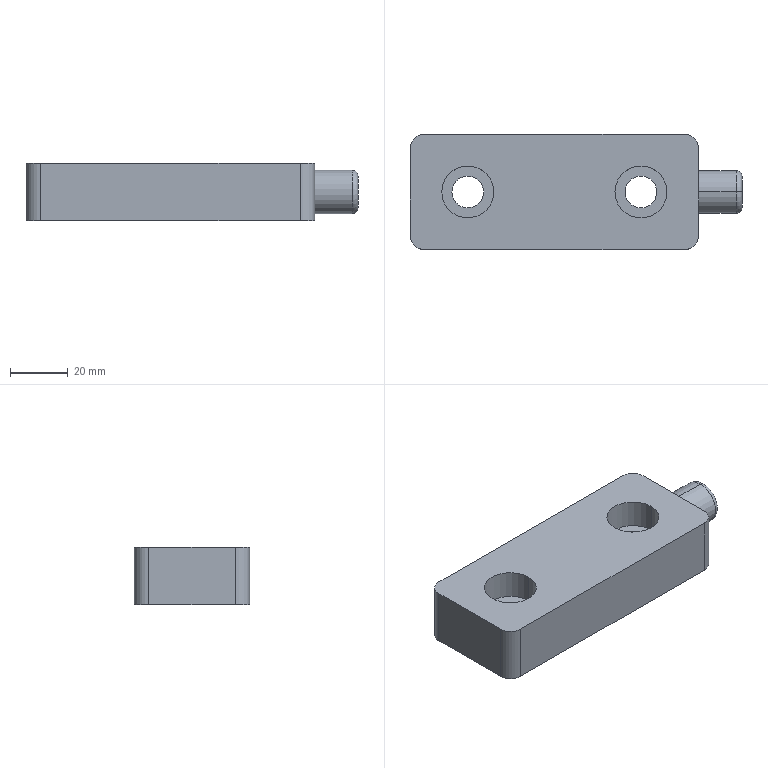Part | SolidWorks | features Fillet 2, ICE 2, Extrusion 1 | 1 solid | 25 faces | box 115 x 40 x 20 mm | volume 75193 mm3 | cylinder 14 | plane 9 | torus 2 | commonest cylinder face diameters 10 x4 11 x4 18 x4 15 x2
STEP:
#1=CARTESIAN_POINT('',(-39.,0.,0.));
#2=VERTEX_POINT('',#1);
#3=CARTESIAN_POINT('',(-21.,0.,0.));
#4=VERTEX_POINT('',#3);
#5=CARTESIAN_POINT('',(-30.,0.,0.));
#6=DIRECTION('',(0.,0.,1.));
#7=DIRECTION('',(1.,0.,0.));
#8=AXIS2_PLACEMENT_3D('',#5,#6,#7);
#9=CIRCLE('',#8,9.);
#10=EDGE_CURVE('',#2,#4,#9,.T.);
#11=ORIENTED_EDGE('',*,*,#10,.F.);
#12=CARTESIAN_POINT('',(-39.,0.,10.));
#13=VERTEX_POINT('',#12);
#14=CARTESIAN_POINT('',(-39.,0.,0.));
#15=DIRECTION('',(0.,0.,1.));
#16=VECTOR('',#15,1000.);
#17=LINE('',#14,#16);
#18=EDGE_CURVE('',#2,#13,#17,.T.);
#19=ORIENTED_EDGE('',*,*,#18,.T.);
#20=CARTESIAN_POINT('',(-21.,0.,10.));
#21=VERTEX_POINT('',#20);
#22=CARTESIAN_POINT('',(-30.,0.,10.));
#23=DIRECTION('',(0.,0.,1.));
#24=DIRECTION('',(1.,0.,0.));
#25=AXIS2_PLACEMENT_3D('',#22,#23,#24);
#26=CIRCLE('',#25,9.);
#27=EDGE_CURVE('',#13,#21,#26,.T.);
#28=ORIENTED_EDGE('',*,*,#27,.T.);
#29=CARTESIAN_POINT('',(-21.,0.,0.));
#30=DIRECTION('',(0.,0.,1.));
#31=VECTOR('',#30,1000.);
#32=LINE('',#29,#31);
#33=EDGE_CURVE('',#4,#21,#32,.T.);
#34=ORIENTED_EDGE('',*,*,#33,.F.);
#35=EDGE_LOOP('',(#11,#19,#28,#34));
#36=FACE_OUTER_BOUND('',#35,.T.);
#37=CARTESIAN_POINT('',(-30.,0.,0.));
#38=DIRECTION('',(0.,0.,1.));
#39=DIRECTION('',(1.,0.,0.));
#40=AXIS2_PLACEMENT_3D('',#37,#38,#39);
#41=CYLINDRICAL_SURFACE('',#40,9.);
#42=ADVANCED_FACE('',(#36),#41,.F.);
#43=CARTESIAN_POINT('',(21.,0.,0.));
#44=VERTEX_POINT('',#43);
#45=CARTESIAN_POINT('',(39.,0.,0.));
#46=VERTEX_POINT('',#45);
#47=CARTESIAN_POINT('',(30.,0.,0.));
#48=DIRECTION('',(0.,0.,1.));
#49=DIRECTION('',(1.,0.,0.));
#50=AXIS2_PLACEMENT_3D('',#47,#48,#49);
#51=CIRCLE('',#50,9.);
#52=EDGE_CURVE('',#44,#46,#51,.T.);
#53=ORIENTED_EDGE('',*,*,#52,.F.);
#54=CARTESIAN_POINT('',(21.,0.,10.));
#55=VERTEX_POINT('',#54);
#56=CARTESIAN_POINT('',(21.,0.,0.));
#57=DIRECTION('',(0.,0.,1.));
#58=VECTOR('',#57,1000.);
#59=LINE('',#56,#58);
#60=EDGE_CURVE('',#44,#55,#59,.T.);
#61=ORIENTED_EDGE('',*,*,#60,.T.);
#62=CARTESIAN_POINT('',(39.,0.,10.));
#63=VERTEX_POINT('',#62);
#64=CARTESIAN_POINT('',(30.,0.,10.));
#65=DIRECTION('',(0.,0.,1.));
#66=DIRECTION('',(1.,0.,0.));
#67=AXIS2_PLACEMENT_3D('',#64,#65,#66);
#68=CIRCLE('',#67,9.);
#69=EDGE_CURVE('',#55,#63,#68,.T.);
#70=ORIENTED_EDGE('',*,*,#69,.T.);
#71=CARTESIAN_POINT('',(39.,0.,0.));
#72=DIRECTION('',(0.,0.,1.));
#73=VECTOR('',#72,1000.);
#74=LINE('',#71,#73);
#75=EDGE_CURVE('',#46,#63,#74,.T.);
#76=ORIENTED_EDGE('',*,*,#75,.F.);
#77=EDGE_LOOP('',(#53,#61,#70,#76));
#78=FACE_OUTER_BOUND('',#77,.T.);
#79=CARTESIAN_POINT('',(30.,0.,0.));
#80=DIRECTION('',(0.,0.,1.));
#81=DIRECTION('',(1.,0.,0.));
#82=AXIS2_PLACEMENT_3D('',#79,#80,#81);
#83=CYLINDRICAL_SURFACE('',#82,9.);
#84=ADVANCED_FACE('',(#78),#83,.F.);
#85=CARTESIAN_POINT('',(63.,0.,7.5));
#86=VERTEX_POINT('',#85);
#87=CARTESIAN_POINT('',(63.,0.,-7.5));
#88=VERTEX_POINT('',#87);
#89=CARTESIAN_POINT('',(63.,0.,0.));
#90=DIRECTION('',(-1.,0.,0.));
#91=DIRECTION('',(0.,0.,-1.));
#92=AXIS2_PLACEMENT_3D('',#89,#90,#91);
#93=CIRCLE('',#92,7.5);
#94=EDGE_CURVE('',#86,#88,#93,.T.);
#95=ORIENTED_EDGE('',*,*,#94,.F.);
#96=CARTESIAN_POINT('',(65.,0.,5.5));
#97=VERTEX_POINT('',#96);
#98=CARTESIAN_POINT('',(63.,0.,5.5));
#99=DIRECTION('',(0.,1.,0.));
#100=DIRECTION('',(0.,0.,1.));
#101=AXIS2_PLACEMENT_3D('',#98,#99,#100);
#102=CIRCLE('',#101,2.);
#103=EDGE_CURVE('',#86,#97,#102,.T.);
#104=ORIENTED_EDGE('',*,*,#103,.T.);
#105=CARTESIAN_POINT('',(65.,0.,-5.5));
#106=VERTEX_POINT('',#105);
#107=CARTESIAN_POINT('',(65.,0.,0.));
#108=DIRECTION('',(1.,0.,0.));
#109=DIRECTION('',(0.,0.,-1.));
#110=AXIS2_PLACEMENT_3D('',#107,#108,#109);
#111=CIRCLE('',#110,5.5);
#112=EDGE_CURVE('',#106,#97,#111,.T.);
#113=ORIENTED_EDGE('',*,*,#112,.F.);
#114=CARTESIAN_POINT('',(63.,0.,-5.5));
#115=DIRECTION('',(0.,-1.,0.));
#116=DIRECTION('',(0.,0.,-1.));
#117=AXIS2_PLACEMENT_3D('',#114,#115,#116);
#118=CIRCLE('',#117,2.);
#119=EDGE_CURVE('',#88,#106,#118,.T.);
#120=ORIENTED_EDGE('',*,*,#119,.F.);
#121=EDGE_LOOP('',(#95,#104,#113,#120));
#122=FACE_OUTER_BOUND('',#121,.T.);
#123=CARTESIAN_POINT('',(63.,0.,0.));
#124=DIRECTION('',(1.,0.,0.));
#125=DIRECTION('',(0.,0.,-1.));
#126=AXIS2_PLACEMENT_3D('',#123,#124,#125);
#127=TOROIDAL_SURFACE('',#126,5.5,2.);
#128=ADVANCED_FACE('',(#122),#127,.T.);
#129=ORIENTED_EDGE('',*,*,#94,.T.);
#130=CARTESIAN_POINT('',(50.,0.,-7.5));
#131=VERTEX_POINT('',#130);
#132=CARTESIAN_POINT('',(65.,0.,-7.5));
#133=DIRECTION('',(-1.,0.,0.));
#134=VECTOR('',#133,1000.);
#135=LINE('',#132,#134);
#136=EDGE_CURVE('',#88,#131,#135,.T.);
#137=ORIENTED_EDGE('',*,*,#136,.T.);
#138=CARTESIAN_POINT('',(50.,0.,7.5));
#139=VERTEX_POINT('',#138);
#140=CARTESIAN_POINT('',(50.,0.,0.));
#141=DIRECTION('',(1.,0.,0.));
#142=DIRECTION('',(0.,0.,-1.));
#143=AXIS2_PLACEMENT_3D('',#140,#141,#142);
#144=CIRCLE('',#143,7.5);
#145=EDGE_CURVE('',#131,#139,#144,.T.);
#146=ORIENTED_EDGE('',*,*,#145,.T.);
#147=CARTESIAN_POINT('',(65.,0.,7.5));
#148=DIRECTION('',(-1.,0.,0.));
#149=VECTOR('',#148,1000.);
#150=LINE('',#147,#149);
#151=EDGE_CURVE('',#86,#139,#150,.T.);
#152=ORIENTED_EDGE('',*,*,#151,.F.);
#153=EDGE_LOOP('',(#129,#137,#146,#152));
#154=FACE_OUTER_BOUND('',#153,.T.);
#155=CARTESIAN_POINT('',(65.,0.,0.));
#156=DIRECTION('',(-1.,0.,0.));
#157=DIRECTION('',(0.,0.,1.));
#158=AXIS2_PLACEMENT_3D('',#155,#156,#157);
#159=CYLINDRICAL_SURFACE('',#158,7.5);
#160=ADVANCED_FACE('',(#154),#159,.T.);
#161=CARTESIAN_POINT('',(24.5,0.,0.));
#162=VERTEX_POINT('',#161);
#163=CARTESIAN_POINT('',(35.5,0.,0.));
#164=VERTEX_POINT('',#163);
#165=CARTESIAN_POINT('',(30.,0.,0.));
#166=DIRECTION('',(0.,0.,1.));
#167=DIRECTION('',(1.,0.,0.));
#168=AXIS2_PLACEMENT_3D('',#165,#166,#167);
#169=CIRCLE('',#168,5.5);
#170=EDGE_CURVE('',#162,#164,#169,.T.);
#171=ORIENTED_EDGE('',*,*,#170,.T.);
#172=CARTESIAN_POINT('',(35.5,0.,-10.));
#173=VERTEX_POINT('',#172);
#174=CARTESIAN_POINT('',(35.5,0.,10.));
#175=DIRECTION('',(0.,0.,-1.));
#176=VECTOR('',#175,1000.);
#177=LINE('',#174,#176);
#178=EDGE_CURVE('',#164,#173,#177,.T.);
#179=ORIENTED_EDGE('',*,*,#178,.T.);
#180=CARTESIAN_POINT('',(24.5,0.,-10.));
#181=VERTEX_POINT('',#180);
#182=CARTESIAN_POINT('',(30.,0.,-10.));
#183=DIRECTION('',(0.,0.,1.));
#184=DIRECTION('',(1.,0.,0.));
#185=AXIS2_PLACEMENT_3D('',#182,#183,#184);
#186=CIRCLE('',#185,5.5);
#187=EDGE_CURVE('',#181,#173,#186,.T.);
#188=ORIENTED_EDGE('',*,*,#187,.F.);
#189=CARTESIAN_POINT('',(24.5,0.,10.));
#190=DIRECTION('',(0.,0.,-1.));
#191=VECTOR('',#190,1000.);
#192=LINE('',#189,#191);
#193=EDGE_CURVE('',#162,#181,#192,.T.);
#194=ORIENTED_EDGE('',*,*,#193,.F.);
#195=EDGE_LOOP('',(#171,#179,#188,#194));
#196=FACE_OUTER_BOUND('',#195,.T.);
#197=CARTESIAN_POINT('',(30.,0.,10.));
#198=DIRECTION('',(0.,0.,-1.));
#199=DIRECTION('',(-1.,0.,0.));
#200=AXIS2_PLACEMENT_3D('',#197,#198,#199);
#201=CYLINDRICAL_SURFACE('',#200,5.5);
#202=ADVANCED_FACE('',(#196),#201,.F.);
#203=CARTESIAN_POINT('',(-35.5,0.,0.));
#204=VERTEX_POINT('',#203);
#205=CARTESIAN_POINT('',(-24.5,0.,0.));
#206=VERTEX_POINT('',#205);
#207=CARTESIAN_POINT('',(-30.,0.,0.));
#208=DIRECTION('',(0.,0.,1.));
#209=DIRECTION('',(1.,0.,0.));
#210=AXIS2_PLACEMENT_3D('',#207,#208,#209);
#211=CIRCLE('',#210,5.5);
#212=EDGE_CURVE('',#204,#206,#211,.T.);
#213=ORIENTED_EDGE('',*,*,#212,.T.);
#214=CARTESIAN_POINT('',(-24.5,0.,-10.));
#215=VERTEX_POINT('',#214);
#216=CARTESIAN_POINT('',(-24.5,0.,10.));
#217=DIRECTION('',(0.,0.,-1.));
#218=VECTOR('',#217,1000.);
#219=LINE('',#216,#218);
#220=EDGE_CURVE('',#206,#215,#219,.T.);
#221=ORIENTED_EDGE('',*,*,#220,.T.);
#222=CARTESIAN_POINT('',(-35.5,0.,-10.));
#223=VERTEX_POINT('',#222);
#224=CARTESIAN_POINT('',(-30.,0.,-10.));
#225=DIRECTION('',(0.,0.,1.));
#226=DIRECTION('',(1.,0.,0.));
#227=AXIS2_PLACEMENT_3D('',#224,#225,#226);
#228=CIRCLE('',#227,5.5);
#229=EDGE_CURVE('',#223,#215,#228,.T.);
#230=ORIENTED_EDGE('',*,*,#229,.F.);
#231=CARTESIAN_POINT('',(-35.5,0.,10.));
#232=DIRECTION('',(0.,0.,-1.));
#233=VECTOR('',#232,1000.);
#234=LINE('',#231,#233);
#235=EDGE_CURVE('',#204,#223,#234,.T.);
#236=ORIENTED_EDGE('',*,*,#235,.F.);
#237=EDGE_LOOP('',(#213,#221,#230,#236));
#238=FACE_OUTER_BOUND('',#237,.T.);
#239=CARTESIAN_POINT('',(-30.,0.,10.));
#240=DIRECTION('',(0.,0.,-1.));
#241=DIRECTION('',(-1.,0.,0.));
#242=AXIS2_PLACEMENT_3D('',#239,#240,#241);
#243=CYLINDRICAL_SURFACE('',#242,5.5);
#244=ADVANCED_FACE('',(#238),#243,.F.);
#245=ORIENTED_EDGE('',*,*,#220,.F.);
#246=CARTESIAN_POINT('',(-30.,0.,0.));
#247=DIRECTION('',(0.,0.,1.));
#248=DIRECTION('',(1.,0.,0.));
#249=AXIS2_PLACEMENT_3D('',#246,#247,#248);
#250=CIRCLE('',#249,5.5);
#251=EDGE_CURVE('',#206,#204,#250,.T.);
#252=ORIENTED_EDGE('',*,*,#251,.T.);
#253=ORIENTED_EDGE('',*,*,#235,.T.);
#254=CARTESIAN_POINT('',(-30.,0.,-10.));
#255=DIRECTION('',(0.,0.,1.));
#256=DIRECTION('',(1.,0.,0.));
#257=AXIS2_PLACEMENT_3D('',#254,#255,#256);
#258=CIRCLE('',#257,5.5);
#259=EDGE_CURVE('',#215,#223,#258,.T.);
#260=ORIENTED_EDGE('',*,*,#259,.F.);
#261=EDGE_LOOP('',(#245,#252,#253,#260));
#262=FACE_OUTER_BOUND('',#261,.T.);
#263=CARTESIAN_POINT('',(-30.,0.,10.));
#264=DIRECTION('',(0.,0.,-1.));
#265=DIRECTION('',(-1.,0.,0.));
#266=AXIS2_PLACEMENT_3D('',#263,#264,#265);
#267=CYLINDRICAL_SURFACE('',#266,5.5);
#268=ADVANCED_FACE('',(#262),#267,.F.);
#269=ORIENTED_EDGE('',*,*,#178,.F.);
#270=CARTESIAN_POINT('',(30.,0.,0.));
#271=DIRECTION('',(0.,0.,1.));
#272=DIRECTION('',(1.,0.,0.));
#273=AXIS2_PLACEMENT_3D('',#270,#271,#272);
#274=CIRCLE('',#273,5.5);
#275=EDGE_CURVE('',#164,#162,#274,.T.);
#276=ORIENTED_EDGE('',*,*,#275,.T.);
#277=ORIENTED_EDGE('',*,*,#193,.T.);
#278=CARTESIAN_POINT('',(30.,0.,-10.));
#279=DIRECTION('',(0.,0.,1.));
#280=DIRECTION('',(1.,0.,0.));
#281=AXIS2_PLACEMENT_3D('',#278,#279,#280);
#282=CIRCLE('',#281,5.5);
#283=EDGE_CURVE('',#173,#181,#282,.T.);
#284=ORIENTED_EDGE('',*,*,#283,.F.);
#285=EDGE_LOOP('',(#269,#276,#277,#284));
#286=FACE_OUTER_BOUND('',#285,.T.);
#287=CARTESIAN_POINT('',(30.,0.,10.));
#288=DIRECTION('',(0.,0.,-1.));
#289=DIRECTION('',(-1.,0.,0.));
#290=AXIS2_PLACEMENT_3D('',#287,#288,#289);
#291=CYLINDRICAL_SURFACE('',#290,5.5);
#292=ADVANCED_FACE('',(#286),#291,.F.);
#293=CARTESIAN_POINT('',(-30.,0.,10.));
#294=DIRECTION('',(0.,0.,1.));
#295=DIRECTION('',(1.,0.,0.));
#296=AXIS2_PLACEMENT_3D('',#293,#294,#295);
#297=CIRCLE('',#296,9.);
#298=EDGE_CURVE('',#21,#13,#297,.T.);
#299=ORIENTED_EDGE('',*,*,#298,.F.);
#300=ORIENTED_EDGE('',*,*,#27,.F.);
#301=EDGE_LOOP('',(#299,#300));
#302=FACE_BOUND('',#301,.T.);
#303=CARTESIAN_POINT('',(30.,0.,10.));
#304=DIRECTION('',(0.,0.,1.));
#305=DIRECTION('',(1.,0.,0.));
#306=AXIS2_PLACEMENT_3D('',#303,#304,#305);
#307=CIRCLE('',#306,9.);
#308=EDGE_CURVE('',#63,#55,#307,.T.);
#309=ORIENTED_EDGE('',*,*,#308,.F.);
#310=ORIENTED_EDGE('',*,*,#69,.F.);
#311=EDGE_LOOP('',(#309,#310));
#312=FACE_BOUND('',#311,.T.);
#313=CARTESIAN_POINT('',(50.,-15.,10.));
#314=VERTEX_POINT('',#313);
#315=CARTESIAN_POINT('',(50.,15.,10.));
#316=VERTEX_POINT('',#315);
#317=CARTESIAN_POINT('',(50.,-20.,10.));
#318=DIRECTION('',(0.,1.,0.));
#319=VECTOR('',#318,1000.);
#320=LINE('',#317,#319);
#321=EDGE_CURVE('',#314,#316,#320,.T.);
#322=ORIENTED_EDGE('',*,*,#321,.T.);
#323=CARTESIAN_POINT('',(45.,20.,10.));
#324=VERTEX_POINT('',#323);
#325=CARTESIAN_POINT('',(45.,15.,10.));
#326=DIRECTION('',(0.,0.,1.));
#327=DIRECTION('',(-1.,0.,0.));
#328=AXIS2_PLACEMENT_3D('',#325,#326,#327);
#329=CIRCLE('',#328,5.);
#330=EDGE_CURVE('',#316,#324,#329,.T.);
#331=ORIENTED_EDGE('',*,*,#330,.T.);
#332=CARTESIAN_POINT('',(-45.,20.,10.));
#333=VERTEX_POINT('',#332);
#334=CARTESIAN_POINT('',(-50.,20.,10.));
#335=DIRECTION('',(-1.,0.,0.));
#336=VECTOR('',#335,1000.);
#337=LINE('',#334,#336);
#338=EDGE_CURVE('',#324,#333,#337,.T.);
#339=ORIENTED_EDGE('',*,*,#338,.T.);
#340=CARTESIAN_POINT('',(-50.,15.,10.));
#341=VERTEX_POINT('',#340);
#342=CARTESIAN_POINT('',(-45.,15.,10.));
#343=DIRECTION('',(0.,0.,1.));
#344=DIRECTION('',(-1.,0.,0.));
#345=AXIS2_PLACEMENT_3D('',#342,#343,#344);
#346=CIRCLE('',#345,5.);
#347=EDGE_CURVE('',#333,#341,#346,.T.);
#348=ORIENTED_EDGE('',*,*,#347,.T.);
#349=CARTESIAN_POINT('',(-50.,-15.,10.));
#350=VERTEX_POINT('',#349);
#351=CARTESIAN_POINT('',(-50.,-20.,10.));
#352=DIRECTION('',(0.,-1.,0.));
#353=VECTOR('',#352,1000.);
#354=LINE('',#351,#353);
#355=EDGE_CURVE('',#341,#350,#354,.T.);
#356=ORIENTED_EDGE('',*,*,#355,.T.);
#357=CARTESIAN_POINT('',(-45.,-20.,10.));
#358=VERTEX_POINT('',#357);
#359=CARTESIAN_POINT('',(-45.,-15.,10.));
#360=DIRECTION('',(0.,0.,1.));
#361=DIRECTION('',(-1.,0.,0.));
#362=AXIS2_PLACEMENT_3D('',#359,#360,#361);
#363=CIRCLE('',#362,5.);
#364=EDGE_CURVE('',#350,#358,#363,.T.);
#365=ORIENTED_EDGE('',*,*,#364,.T.);
#366=CARTESIAN_POINT('',(45.,-20.,10.));
#367=VERTEX_POINT('',#366);
#368=CARTESIAN_POINT('',(-50.,-20.,10.));
#369=DIRECTION('',(1.,0.,0.));
#370=VECTOR('',#369,1000.);
#371=LINE('',#368,#370);
#372=EDGE_CURVE('',#358,#367,#371,.T.);
#373=ORIENTED_EDGE('',*,*,#372,.T.);
#374=CARTESIAN_POINT('',(45.,-15.,10.));
#375=DIRECTION('',(0.,0.,1.));
#376=DIRECTION('',(-1.,0.,0.));
#377=AXIS2_PLACEMENT_3D('',#374,#375,#376);
#378=CIRCLE('',#377,5.);
#379=EDGE_CURVE('',#367,#314,#378,.T.);
#380=ORIENTED_EDGE('',*,*,#379,.T.);
#381=EDGE_LOOP('',(#322,#331,#339,#348,#356,#365,#373,#380));
#382=FACE_OUTER_BOUND('',#381,.T.);
#383=CARTESIAN_POINT('',(0.,0.,10.));
#384=DIRECTION('',(0.,0.,-1.));
#385=DIRECTION('',(-1.,0.,0.));
#386=AXIS2_PLACEMENT_3D('',#383,#384,#385);
#387=PLANE('',#386);
#388=ADVANCED_FACE('',(#302,#312,#382),#387,.F.);
#389=ORIENTED_EDGE('',*,*,#229,.T.);
#390=ORIENTED_EDGE('',*,*,#259,.T.);
#391=EDGE_LOOP('',(#389,#390));
#392=FACE_BOUND('',#391,.T.);
#393=CARTESIAN_POINT('',(45.,20.,-10.));
#394=VERTEX_POINT('',#393);
#395=CARTESIAN_POINT('',(-45.,20.,-10.));
#396=VERTEX_POINT('',#395);
#397=CARTESIAN_POINT('',(-50.,20.,-10.));
#398=DIRECTION('',(-1.,0.,0.));
#399=VECTOR('',#398,1000.);
#400=LINE('',#397,#399);
#401=EDGE_CURVE('',#394,#396,#400,.T.);
#402=ORIENTED_EDGE('',*,*,#401,.F.);
#403=CARTESIAN_POINT('',(50.,15.,-10.));
#404=VERTEX_POINT('',#403);
#405=CARTESIAN_POINT('',(45.,15.,-10.));
#406=DIRECTION('',(0.,0.,-1.));
#407=DIRECTION('',(-1.,0.,0.));
#408=AXIS2_PLACEMENT_3D('',#405,#406,#407);
#409=CIRCLE('',#408,5.);
#410=EDGE_CURVE('',#394,#404,#409,.T.);
#411=ORIENTED_EDGE('',*,*,#410,.T.);
#412=CARTESIAN_POINT('',(50.,-15.,-10.));
#413=VERTEX_POINT('',#412);
#414=CARTESIAN_POINT('',(50.,-20.,-10.));
#415=DIRECTION('',(0.,1.,0.));
#416=VECTOR('',#415,1000.);
#417=LINE('',#414,#416);
#418=EDGE_CURVE('',#413,#404,#417,.T.);
#419=ORIENTED_EDGE('',*,*,#418,.F.);
#420=CARTESIAN_POINT('',(45.,-20.,-10.));
#421=VERTEX_POINT('',#420);
#422=CARTESIAN_POINT('',(45.,-15.,-10.));
#423=DIRECTION('',(0.,0.,-1.));
#424=DIRECTION('',(-1.,0.,0.));
#425=AXIS2_PLACEMENT_3D('',#422,#423,#424);
#426=CIRCLE('',#425,5.);
#427=EDGE_CURVE('',#413,#421,#426,.T.);
#428=ORIENTED_EDGE('',*,*,#427,.T.);
#429=CARTESIAN_POINT('',(-45.,-20.,-10.));
#430=VERTEX_POINT('',#429);
#431=CARTESIAN_POINT('',(-50.,-20.,-10.));
#432=DIRECTION('',(1.,0.,0.));
#433=VECTOR('',#432,1000.);
#434=LINE('',#431,#433);
#435=EDGE_CURVE('',#430,#421,#434,.T.);
#436=ORIENTED_EDGE('',*,*,#435,.F.);
#437=CARTESIAN_POINT('',(-50.,-15.,-10.));
#438=VERTEX_POINT('',#437);
#439=CARTESIAN_POINT('',(-45.,-15.,-10.));
#440=DIRECTION('',(0.,0.,-1.));
#441=DIRECTION('',(-1.,0.,0.));
#442=AXIS2_PLACEMENT_3D('',#439,#440,#441);
#443=CIRCLE('',#442,5.);
#444=EDGE_CURVE('',#430,#438,#443,.T.);
#445=ORIENTED_EDGE('',*,*,#444,.T.);
#446=CARTESIAN_POINT('',(-50.,15.,-10.));
#447=VERTEX_POINT('',#446);
#448=CARTESIAN_POINT('',(-50.,-20.,-10.));
#449=DIRECTION('',(0.,-1.,0.));
#450=VECTOR('',#449,1000.);
#451=LINE('',#448,#450);
#452=EDGE_CURVE('',#447,#438,#451,.T.);
#453=ORIENTED_EDGE('',*,*,#452,.F.);
#454=CARTESIAN_POINT('',(-45.,15.,-10.));
#455=DIRECTION('',(0.,0.,-1.));
#456=DIRECTION('',(-1.,0.,0.));
#457=AXIS2_PLACEMENT_3D('',#454,#455,#456);
#458=CIRCLE('',#457,5.);
#459=EDGE_CURVE('',#447,#396,#458,.T.);
#460=ORIENTED_EDGE('',*,*,#459,.T.);
#461=EDGE_LOOP('',(#402,#411,#419,#428,#436,#445,#453,#460));
#462=FACE_OUTER_BOUND('',#461,.T.);
#463=ORIENTED_EDGE('',*,*,#187,.T.);
#464=ORIENTED_EDGE('',*,*,#283,.T.);
#465=EDGE_LOOP('',(#463,#464));
#466=FACE_BOUND('',#465,.T.);
#467=CARTESIAN_POINT('',(0.,0.,-10.));
#468=DIRECTION('',(0.,0.,-1.));
#469=DIRECTION('',(-1.,0.,0.));
#470=AXIS2_PLACEMENT_3D('',#467,#468,#469);
#471=PLANE('',#470);
#472=ADVANCED_FACE('',(#392,#462,#466),#471,.T.);
#473=CARTESIAN_POINT('',(50.,0.,0.));
#474=DIRECTION('',(1.,0.,0.));
#475=DIRECTION('',(0.,0.,-1.));
#476=AXIS2_PLACEMENT_3D('',#473,#474,#475);
#477=CIRCLE('',#476,7.5);
#478=EDGE_CURVE('',#139,#131,#477,.T.);
#479=ORIENTED_EDGE('',*,*,#478,.F.);
#480=ORIENTED_EDGE('',*,*,#145,.F.);
#481=EDGE_LOOP('',(#479,#480));
#482=FACE_BOUND('',#481,.T.);
#483=ORIENTED_EDGE('',*,*,#418,.T.);
#484=CARTESIAN_POINT('',(50.,15.,10.));
#485=DIRECTION('',(0.,0.,1.));
#486=VECTOR('',#485,1000.);
#487=LINE('',#484,#486);
#488=EDGE_CURVE('',#404,#316,#487,.T.);
#489=ORIENTED_EDGE('',*,*,#488,.T.);
#490=ORIENTED_EDGE('',*,*,#321,.F.);
#491=CARTESIAN_POINT('',(50.,-15.,10.));
#492=DIRECTION('',(0.,0.,-1.));
#493=VECTOR('',#492,1000.);
#494=LINE('',#491,#493);
#495=EDGE_CURVE('',#314,#413,#494,.T.);
#496=ORIENTED_EDGE('',*,*,#495,.T.);
#497=EDGE_LOOP('',(#483,#489,#490,#496));
#498=FACE_OUTER_BOUND('',#497,.T.);
#499=CARTESIAN_POINT('',(50.,-20.,10.));
#500=DIRECTION('',(-1.,0.,0.));
#501=DIRECTION('',(0.,0.,1.));
#502=AXIS2_PLACEMENT_3D('',#499,#500,#501);
#503=PLANE('',#502);
#504=ADVANCED_FACE('',(#482,#498),#503,.F.);
#505=ORIENTED_EDGE('',*,*,#338,.F.);
#506=CARTESIAN_POINT('',(45.,20.,10.));
#507=DIRECTION('',(0.,0.,-1.));
#508=VECTOR('',#507,1000.);
#509=LINE('',#506,#508);
#510=EDGE_CURVE('',#324,#394,#509,.T.);
#511=ORIENTED_EDGE('',*,*,#510,.T.);
#512=ORIENTED_EDGE('',*,*,#401,.T.);
#513=CARTESIAN_POINT('',(-45.,20.,10.));
#514=DIRECTION('',(0.,0.,1.));
#515=VECTOR('',#514,1000.);
#516=LINE('',#513,#515);
#517=EDGE_CURVE('',#396,#333,#516,.T.);
#518=ORIENTED_EDGE('',*,*,#517,.T.);
#519=EDGE_LOOP('',(#505,#511,#512,#518));
#520=FACE_OUTER_BOUND('',#519,.T.);
#521=CARTESIAN_POINT('',(-50.,20.,10.));
#522=DIRECTION('',(0.,-1.,0.));
#523=DIRECTION('',(0.,0.,-1.));
#524=AXIS2_PLACEMENT_3D('',#521,#522,#523);
#525=PLANE('',#524);
#526=ADVANCED_FACE('',(#520),#525,.F.);
#527=ORIENTED_EDGE('',*,*,#452,.T.);
#528=CARTESIAN_POINT('',(-50.,-15.,10.));
#529=DIRECTION('',(0.,0.,1.));
#530=VECTOR('',#529,1000.);
#531=LINE('',#528,#530);
#532=EDGE_CURVE('',#438,#350,#531,.T.);
#533=ORIENTED_EDGE('',*,*,#532,.T.);
#534=ORIENTED_EDGE('',*,*,#355,.F.);
#535=CARTESIAN_POINT('',(-50.,15.,10.));
#536=DIRECTION('',(0.,0.,-1.));
#537=VECTOR('',#536,1000.);
#538=LINE('',#535,#537);
#539=EDGE_CURVE('',#341,#447,#538,.T.);
#540=ORIENTED_EDGE('',*,*,#539,.T.);
#541=EDGE_LOOP('',(#527,#533,#534,#540));
#542=FACE_OUTER_BOUND('',#541,.T.);
#543=CARTESIAN_POINT('',(-50.,-20.,10.));
#544=DIRECTION('',(1.,0.,0.));
#545=DIRECTION('',(0.,0.,-1.));
#546=AXIS2_PLACEMENT_3D('',#543,#544,#545);
#547=PLANE('',#546);
#548=ADVANCED_FACE('',(#542),#547,.F.);
#549=ORIENTED_EDGE('',*,*,#435,.T.);
#550=CARTESIAN_POINT('',(45.,-20.,10.));
#551=DIRECTION('',(0.,0.,1.));
#552=VECTOR('',#551,1000.);
#553=LINE('',#550,#552);
#554=EDGE_CURVE('',#421,#367,#553,.T.);
#555=ORIENTED_EDGE('',*,*,#554,.T.);
#556=ORIENTED_EDGE('',*,*,#372,.F.);
#557=CARTESIAN_POINT('',(-45.,-20.,10.));
#558=DIRECTION('',(0.,0.,-1.));
#559=VECTOR('',#558,1000.);
#560=LINE('',#557,#559);
#561=EDGE_CURVE('',#358,#430,#560,.T.);
#562=ORIENTED_EDGE('',*,*,#561,.T.);
#563=EDGE_LOOP('',(#549,#555,#556,#562));
#564=FACE_OUTER_BOUND('',#563,.T.);
#565=CARTESIAN_POINT('',(-50.,-20.,10.));
#566=DIRECTION('',(0.,1.,0.));
#567=DIRECTION('',(0.,0.,1.));
#568=AXIS2_PLACEMENT_3D('',#565,#566,#567);
#569=PLANE('',#568);
#570=ADVANCED_FACE('',(#564),#569,.F.);
#571=ORIENTED_EDGE('',*,*,#136,.F.);
#572=CARTESIAN_POINT('',(63.,0.,0.));
#573=DIRECTION('',(-1.,0.,0.));
#574=DIRECTION('',(0.,0.,-1.));
#575=AXIS2_PLACEMENT_3D('',#572,#573,#574);
#576=CIRCLE('',#575,7.5);
#577=EDGE_CURVE('',#88,#86,#576,.T.);
#578=ORIENTED_EDGE('',*,*,#577,.T.);
#579=ORIENTED_EDGE('',*,*,#151,.T.);
#580=ORIENTED_EDGE('',*,*,#478,.T.);
#581=EDGE_LOOP('',(#571,#578,#579,#580));
#582=FACE_OUTER_BOUND('',#581,.T.);
#583=CARTESIAN_POINT('',(65.,0.,0.));
#584=DIRECTION('',(-1.,0.,0.));
#585=DIRECTION('',(0.,0.,1.));
#586=AXIS2_PLACEMENT_3D('',#583,#584,#585);
#587=CYLINDRICAL_SURFACE('',#586,7.5);
#588=ADVANCED_FACE('',(#582),#587,.T.);
#589=ORIENTED_EDGE('',*,*,#112,.T.);
#590=CARTESIAN_POINT('',(65.,0.,0.));
#591=DIRECTION('',(1.,0.,0.));
#592=DIRECTION('',(0.,0.,-1.));
#593=AXIS2_PLACEMENT_3D('',#590,#591,#592);
#594=CIRCLE('',#593,5.5);
#595=EDGE_CURVE('',#97,#106,#594,.T.);
#596=ORIENTED_EDGE('',*,*,#595,.T.);
#597=EDGE_LOOP('',(#589,#596));
#598=FACE_OUTER_BOUND('',#597,.T.);
#599=CARTESIAN_POINT('',(65.,0.,0.));
#600=DIRECTION('',(1.,0.,0.));
#601=DIRECTION('',(0.,0.,-1.));
#602=AXIS2_PLACEMENT_3D('',#599,#600,#601);
#603=PLANE('',#602);
#604=ADVANCED_FACE('',(#598),#603,.T.);
#605=ORIENTED_EDGE('',*,*,#103,.F.);
#606=ORIENTED_EDGE('',*,*,#577,.F.);
#607=ORIENTED_EDGE('',*,*,#119,.T.);
#608=ORIENTED_EDGE('',*,*,#595,.F.);
#609=EDGE_LOOP('',(#605,#606,#607,#608));
#610=FACE_OUTER_BOUND('',#609,.T.);
#611=CARTESIAN_POINT('',(63.,0.,0.));
#612=DIRECTION('',(1.,0.,0.));
#613=DIRECTION('',(0.,0.,-1.));
#614=AXIS2_PLACEMENT_3D('',#611,#612,#613);
#615=TOROIDAL_SURFACE('',#614,5.5,2.);
#616=ADVANCED_FACE('',(#610),#615,.T.);
#617=ORIENTED_EDGE('',*,*,#60,.F.);
#618=CARTESIAN_POINT('',(30.,0.,0.));
#619=DIRECTION('',(0.,0.,1.));
#620=DIRECTION('',(1.,0.,0.));
#621=AXIS2_PLACEMENT_3D('',#618,#619,#620);
#622=CIRCLE('',#621,9.);
#623=EDGE_CURVE('',#46,#44,#622,.T.);
#624=ORIENTED_EDGE('',*,*,#623,.F.);
#625=ORIENTED_EDGE('',*,*,#75,.T.);
#626=ORIENTED_EDGE('',*,*,#308,.T.);
#627=EDGE_LOOP('',(#617,#624,#625,#626));
#628=FACE_OUTER_BOUND('',#627,.T.);
#629=CARTESIAN_POINT('',(30.,0.,0.));
#630=DIRECTION('',(0.,0.,1.));
#631=DIRECTION('',(1.,0.,0.));
#632=AXIS2_PLACEMENT_3D('',#629,#630,#631);
#633=CYLINDRICAL_SURFACE('',#632,9.);
#634=ADVANCED_FACE('',(#628),#633,.F.);
#635=ORIENTED_EDGE('',*,*,#170,.F.);
#636=ORIENTED_EDGE('',*,*,#275,.F.);
#637=EDGE_LOOP('',(#635,#636));
#638=FACE_BOUND('',#637,.T.);
#639=ORIENTED_EDGE('',*,*,#623,.T.);
#640=ORIENTED_EDGE('',*,*,#52,.T.);
#641=EDGE_LOOP('',(#639,#640));
#642=FACE_OUTER_BOUND('',#641,.T.);
#643=CARTESIAN_POINT('',(30.,0.,0.));
#644=DIRECTION('',(0.,0.,1.));
#645=DIRECTION('',(1.,0.,0.));
#646=AXIS2_PLACEMENT_3D('',#643,#644,#645);
#647=PLANE('',#646);
#648=ADVANCED_FACE('',(#638,#642),#647,.T.);
#649=ORIENTED_EDGE('',*,*,#18,.F.);
#650=CARTESIAN_POINT('',(-30.,0.,0.));
#651=DIRECTION('',(0.,0.,1.));
#652=DIRECTION('',(1.,0.,0.));
#653=AXIS2_PLACEMENT_3D('',#650,#651,#652);
#654=CIRCLE('',#653,9.);
#655=EDGE_CURVE('',#4,#2,#654,.T.);
#656=ORIENTED_EDGE('',*,*,#655,.F.);
#657=ORIENTED_EDGE('',*,*,#33,.T.);
#658=ORIENTED_EDGE('',*,*,#298,.T.);
#659=EDGE_LOOP('',(#649,#656,#657,#658));
#660=FACE_OUTER_BOUND('',#659,.T.);
#661=CARTESIAN_POINT('',(-30.,0.,0.));
#662=DIRECTION('',(0.,0.,1.));
#663=DIRECTION('',(1.,0.,0.));
#664=AXIS2_PLACEMENT_3D('',#661,#662,#663);
#665=CYLINDRICAL_SURFACE('',#664,9.);
#666=ADVANCED_FACE('',(#660),#665,.F.);
#667=ORIENTED_EDGE('',*,*,#212,.F.);
#668=ORIENTED_EDGE('',*,*,#251,.F.);
#669=EDGE_LOOP('',(#667,#668));
#670=FACE_BOUND('',#669,.T.);
#671=ORIENTED_EDGE('',*,*,#655,.T.);
#672=ORIENTED_EDGE('',*,*,#10,.T.);
#673=EDGE_LOOP('',(#671,#672));
#674=FACE_OUTER_BOUND('',#673,.T.);
#675=CARTESIAN_POINT('',(-30.,0.,0.));
#676=DIRECTION('',(0.,0.,1.));
#677=DIRECTION('',(1.,0.,0.));
#678=AXIS2_PLACEMENT_3D('',#675,#676,#677);
#679=PLANE('',#678);
#680=ADVANCED_FACE('',(#670,#674),#679,.T.);
#681=ORIENTED_EDGE('',*,*,#330,.F.);
#682=ORIENTED_EDGE('',*,*,#488,.F.);
#683=ORIENTED_EDGE('',*,*,#410,.F.);
#684=ORIENTED_EDGE('',*,*,#510,.F.);
#685=EDGE_LOOP('',(#681,#682,#683,#684));
#686=FACE_OUTER_BOUND('',#685,.T.);
#687=CARTESIAN_POINT('',(45.,15.,10.));
#688=DIRECTION('',(0.,0.,-1.));
#689=DIRECTION('',(-1.,0.,0.));
#690=AXIS2_PLACEMENT_3D('',#687,#688,#689);
#691=CYLINDRICAL_SURFACE('',#690,5.);
#692=ADVANCED_FACE('',(#686),#691,.T.);
#693=ORIENTED_EDGE('',*,*,#379,.F.);
#694=ORIENTED_EDGE('',*,*,#554,.F.);
#695=ORIENTED_EDGE('',*,*,#427,.F.);
#696=ORIENTED_EDGE('',*,*,#495,.F.);
#697=EDGE_LOOP('',(#693,#694,#695,#696));
#698=FACE_OUTER_BOUND('',#697,.T.);
#699=CARTESIAN_POINT('',(45.,-15.,10.));
#700=DIRECTION('',(0.,0.,-1.));
#701=DIRECTION('',(-1.,0.,0.));
#702=AXIS2_PLACEMENT_3D('',#699,#700,#701);
#703=CYLINDRICAL_SURFACE('',#702,5.);
#704=ADVANCED_FACE('',(#698),#703,.T.);
#705=ORIENTED_EDGE('',*,*,#364,.F.);
#706=ORIENTED_EDGE('',*,*,#532,.F.);
#707=ORIENTED_EDGE('',*,*,#444,.F.);
#708=ORIENTED_EDGE('',*,*,#561,.F.);
#709=EDGE_LOOP('',(#705,#706,#707,#708));
#710=FACE_OUTER_BOUND('',#709,.T.);
#711=CARTESIAN_POINT('',(-45.,-15.,10.));
#712=DIRECTION('',(0.,0.,-1.));
#713=DIRECTION('',(-1.,0.,0.));
#714=AXIS2_PLACEMENT_3D('',#711,#712,#713);
#715=CYLINDRICAL_SURFACE('',#714,5.);
#716=ADVANCED_FACE('',(#710),#715,.T.);
#717=ORIENTED_EDGE('',*,*,#347,.F.);
#718=ORIENTED_EDGE('',*,*,#517,.F.);
#719=ORIENTED_EDGE('',*,*,#459,.F.);
#720=ORIENTED_EDGE('',*,*,#539,.F.);
#721=EDGE_LOOP('',(#717,#718,#719,#720));
#722=FACE_OUTER_BOUND('',#721,.T.);
#723=CARTESIAN_POINT('',(-45.,15.,10.));
#724=DIRECTION('',(0.,0.,-1.));
#725=DIRECTION('',(-1.,0.,0.));
#726=AXIS2_PLACEMENT_3D('',#723,#724,#725);
#727=CYLINDRICAL_SURFACE('',#726,5.);
#728=ADVANCED_FACE('',(#722),#727,.T.);
#729=CLOSED_SHELL('',(#42,#84,#128,#160,#202,#244,#268,#292,#388,#472,#504,#526,#548,#570,#588,#604,#616,#634,#648,#666,#680,#692,#704,#716,#728));
#730=MANIFOLD_SOLID_BREP('',#729);
#731=CARTESIAN_POINT('',(0.,0.,0.));
#732=DIRECTION('',(0.,0.,1.));
#733=DIRECTION('',(1.,0.,0.));
#734=AXIS2_PLACEMENT_3D('',#731,#732,#733);
#735=(LENGTH_UNIT()NAMED_UNIT(*)SI_UNIT(.MILLI.,.METRE.));
#736=UNCERTAINTY_MEASURE_WITH_UNIT(LENGTH_MEASURE(0.00001),#735,'','');
#737=(NAMED_UNIT(*)PLANE_ANGLE_UNIT()SI_UNIT($,.RADIAN.));
#738=(NAMED_UNIT(*)SI_UNIT($,.STERADIAN.)SOLID_ANGLE_UNIT());
#739=(GEOMETRIC_REPRESENTATION_CONTEXT(3)GLOBAL_UNCERTAINTY_ASSIGNED_CONTEXT((#736))GLOBAL_UNIT_ASSIGNED_CONTEXT((#735,#737,#738))REPRESENTATION_CONTEXT('',''));
#740=ADVANCED_BREP_SHAPE_REPRESENTATION('',(#730,#734),#739);